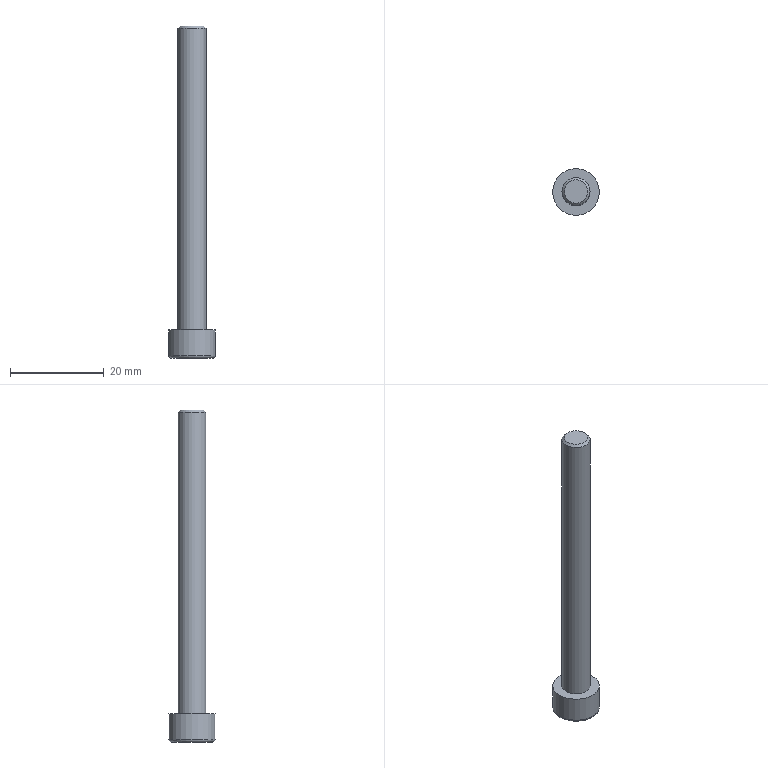Part | NX | features solid 2 | 1 solid | 14 faces | box 10 x 10 x 71 mm | volume 2240 mm3 | plane 10 | cylinder 2 | torus 1 | cone 1 | commonest cylinder face diameters 6 x1 10 x1
STEP:
#1=CARTESIAN_POINT('',(-100.557,-105.5,-189.5));
#2=VERTEX_POINT('',#1);
#3=CARTESIAN_POINT('',(-99.113,-108.,-189.5));
#4=VERTEX_POINT('',#3);
#5=CARTESIAN_POINT('',(-100.557,-105.5,-189.5));
#6=DIRECTION('',(0.5,-0.866,0.));
#7=VECTOR('',#6,1000.);
#8=LINE('',#5,#7);
#9=EDGE_CURVE('',#2,#4,#8,.T.);
#10=ORIENTED_EDGE('',*,*,#9,.F.);
#11=CARTESIAN_POINT('',(-103.443,-105.5,-189.5));
#12=VERTEX_POINT('',#11);
#13=CARTESIAN_POINT('',(-103.443,-105.5,-189.5));
#14=DIRECTION('',(1.,0.,0.));
#15=VECTOR('',#14,1000.);
#16=LINE('',#13,#15);
#17=EDGE_CURVE('',#12,#2,#16,.T.);
#18=ORIENTED_EDGE('',*,*,#17,.F.);
#19=CARTESIAN_POINT('',(-104.887,-108.,-189.5));
#20=VERTEX_POINT('',#19);
#21=CARTESIAN_POINT('',(-104.887,-108.,-189.5));
#22=DIRECTION('',(0.5,0.866,0.));
#23=VECTOR('',#22,1000.);
#24=LINE('',#21,#23);
#25=EDGE_CURVE('',#20,#12,#24,.T.);
#26=ORIENTED_EDGE('',*,*,#25,.F.);
#27=CARTESIAN_POINT('',(-103.443,-110.5,-189.5));
#28=VERTEX_POINT('',#27);
#29=CARTESIAN_POINT('',(-103.443,-110.5,-189.5));
#30=DIRECTION('',(-0.5,0.866,0.));
#31=VECTOR('',#30,1000.);
#32=LINE('',#29,#31);
#33=EDGE_CURVE('',#28,#20,#32,.T.);
#34=ORIENTED_EDGE('',*,*,#33,.F.);
#35=CARTESIAN_POINT('',(-100.557,-110.5,-189.5));
#36=VERTEX_POINT('',#35);
#37=CARTESIAN_POINT('',(-100.557,-110.5,-189.5));
#38=DIRECTION('',(-1.,0.,0.));
#39=VECTOR('',#38,1000.);
#40=LINE('',#37,#39);
#41=EDGE_CURVE('',#36,#28,#40,.T.);
#42=ORIENTED_EDGE('',*,*,#41,.F.);
#43=CARTESIAN_POINT('',(-99.113,-108.,-189.5));
#44=DIRECTION('',(-0.5,-0.866,0.));
#45=VECTOR('',#44,1000.);
#46=LINE('',#43,#45);
#47=EDGE_CURVE('',#4,#36,#46,.T.);
#48=ORIENTED_EDGE('',*,*,#47,.F.);
#49=EDGE_LOOP('',(#10,#18,#26,#34,#42,#48));
#50=FACE_BOUND('',#49,.T.);
#51=CARTESIAN_POINT('',(-106.5,-108.,-189.5));
#52=VERTEX_POINT('',#51);
#53=CARTESIAN_POINT('',(-102.,-108.,-189.5));
#54=DIRECTION('',(0.,0.,-1.));
#55=DIRECTION('',(-1.,0.,0.));
#56=AXIS2_PLACEMENT_3D('',#53,#54,#55);
#57=CIRCLE('',#56,4.5);
#58=EDGE_CURVE('',#52,#52,#57,.T.);
#59=ORIENTED_EDGE('',*,*,#58,.T.);
#60=EDGE_LOOP('',(#59));
#61=FACE_BOUND('',#60,.T.);
#62=CARTESIAN_POINT('',(-102.,-108.,-189.5));
#63=DIRECTION('',(0.,0.,-1.));
#64=DIRECTION('',(-1.,0.,0.));
#65=AXIS2_PLACEMENT_3D('',#62,#63,#64);
#66=PLANE('',#65);
#67=ADVANCED_FACE('',(#50,#61),#66,.T.);
#68=CARTESIAN_POINT('',(-99.,-108.,-183.5));
#69=VERTEX_POINT('',#68);
#70=CARTESIAN_POINT('',(-102.,-108.,-183.5));
#71=DIRECTION('',(0.,0.,1.));
#72=DIRECTION('',(1.,0.,0.));
#73=AXIS2_PLACEMENT_3D('',#70,#71,#72);
#74=CIRCLE('',#73,3.);
#75=EDGE_CURVE('',#69,#69,#74,.T.);
#76=ORIENTED_EDGE('',*,*,#75,.F.);
#77=EDGE_LOOP('',(#76));
#78=FACE_BOUND('',#77,.T.);
#79=CARTESIAN_POINT('',(-97.,-108.,-183.5));
#80=VERTEX_POINT('',#79);
#81=CARTESIAN_POINT('',(-102.,-108.,-183.5));
#82=DIRECTION('',(0.,0.,-1.));
#83=DIRECTION('',(1.,0.,0.));
#84=AXIS2_PLACEMENT_3D('',#81,#82,#83);
#85=CIRCLE('',#84,5.);
#86=EDGE_CURVE('',#80,#80,#85,.T.);
#87=ORIENTED_EDGE('',*,*,#86,.F.);
#88=EDGE_LOOP('',(#87));
#89=FACE_BOUND('',#88,.T.);
#90=CARTESIAN_POINT('',(-102.,-108.,-183.5));
#91=DIRECTION('',(0.,0.,1.));
#92=DIRECTION('',(1.,0.,0.));
#93=AXIS2_PLACEMENT_3D('',#90,#91,#92);
#94=PLANE('',#93);
#95=ADVANCED_FACE('',(#78,#89),#94,.T.);
#96=CARTESIAN_POINT('',(-107.,-108.,-189.));
#97=VERTEX_POINT('',#96);
#98=CARTESIAN_POINT('',(-102.,-108.,-189.));
#99=DIRECTION('',(0.,0.,-1.));
#100=DIRECTION('',(-1.,0.,0.));
#101=AXIS2_PLACEMENT_3D('',#98,#99,#100);
#102=CIRCLE('',#101,5.);
#103=EDGE_CURVE('',#97,#97,#102,.F.);
#104=ORIENTED_EDGE('',*,*,#103,.T.);
#105=EDGE_LOOP('',(#104));
#106=FACE_BOUND('',#105,.T.);
#107=ORIENTED_EDGE('',*,*,#86,.T.);
#108=EDGE_LOOP('',(#107));
#109=FACE_BOUND('',#108,.T.);
#110=CARTESIAN_POINT('',(-102.,-108.,-183.5));
#111=DIRECTION('',(0.,0.,-1.));
#112=DIRECTION('',(1.,0.,0.));
#113=AXIS2_PLACEMENT_3D('',#110,#111,#112);
#114=CYLINDRICAL_SURFACE('',#113,5.);
#115=ADVANCED_FACE('',(#106,#109),#114,.T.);
#116=ORIENTED_EDGE('',*,*,#58,.F.);
#117=EDGE_LOOP('',(#116));
#118=FACE_BOUND('',#117,.T.);
#119=ORIENTED_EDGE('',*,*,#103,.F.);
#120=EDGE_LOOP('',(#119));
#121=FACE_BOUND('',#120,.T.);
#122=CARTESIAN_POINT('',(-102.,-108.,-189.));
#123=DIRECTION('',(0.,0.,-1.));
#124=DIRECTION('',(-1.,0.,0.));
#125=AXIS2_PLACEMENT_3D('',#122,#123,#124);
#126=TOROIDAL_SURFACE('',#125,4.5,0.5);
#127=ADVANCED_FACE('',(#118,#121),#126,.T.);
#128=CARTESIAN_POINT('',(-99.5,-108.,-118.5));
#129=VERTEX_POINT('',#128);
#130=CARTESIAN_POINT('',(-102.,-108.,-118.5));
#131=DIRECTION('',(0.,0.,1.));
#132=DIRECTION('',(1.,0.,0.));
#133=AXIS2_PLACEMENT_3D('',#130,#131,#132);
#134=CIRCLE('',#133,2.5);
#135=EDGE_CURVE('',#129,#129,#134,.T.);
#136=ORIENTED_EDGE('',*,*,#135,.T.);
#137=EDGE_LOOP('',(#136));
#138=FACE_BOUND('',#137,.T.);
#139=CARTESIAN_POINT('',(-102.,-108.,-118.5));
#140=DIRECTION('',(0.,0.,1.));
#141=DIRECTION('',(1.,0.,0.));
#142=AXIS2_PLACEMENT_3D('',#139,#140,#141);
#143=PLANE('',#142);
#144=ADVANCED_FACE('',(#138),#143,.T.);
#145=CARTESIAN_POINT('',(-99.,-108.,-119.));
#146=VERTEX_POINT('',#145);
#147=CARTESIAN_POINT('',(-102.,-108.,-119.));
#148=DIRECTION('',(0.,0.,1.));
#149=DIRECTION('',(1.,0.,0.));
#150=AXIS2_PLACEMENT_3D('',#147,#148,#149);
#151=CIRCLE('',#150,3.);
#152=EDGE_CURVE('',#146,#146,#151,.F.);
#153=ORIENTED_EDGE('',*,*,#152,.T.);
#154=EDGE_LOOP('',(#153));
#155=FACE_BOUND('',#154,.T.);
#156=ORIENTED_EDGE('',*,*,#75,.T.);
#157=EDGE_LOOP('',(#156));
#158=FACE_BOUND('',#157,.T.);
#159=CARTESIAN_POINT('',(-102.,-108.,-118.5));
#160=DIRECTION('',(0.,0.,-1.));
#161=DIRECTION('',(1.,0.,0.));
#162=AXIS2_PLACEMENT_3D('',#159,#160,#161);
#163=CYLINDRICAL_SURFACE('',#162,3.);
#164=ADVANCED_FACE('',(#155,#158),#163,.T.);
#165=ORIENTED_EDGE('',*,*,#135,.F.);
#166=EDGE_LOOP('',(#165));
#167=FACE_BOUND('',#166,.T.);
#168=ORIENTED_EDGE('',*,*,#152,.F.);
#169=EDGE_LOOP('',(#168));
#170=FACE_BOUND('',#169,.T.);
#171=CARTESIAN_POINT('',(-102.,-108.,-119.));
#172=DIRECTION('',(0.,0.,-1.));
#173=DIRECTION('',(-1.,0.,0.));
#174=AXIS2_PLACEMENT_3D('',#171,#172,#173);
#175=CONICAL_SURFACE('',#174,3.,0.7854);
#176=ADVANCED_FACE('',(#167,#170),#175,.T.);
#177=ORIENTED_EDGE('',*,*,#9,.T.);
#178=CARTESIAN_POINT('',(-99.113,-108.,-186.5));
#179=VERTEX_POINT('',#178);
#180=CARTESIAN_POINT('',(-99.113,-108.,-186.5));
#181=DIRECTION('',(0.,0.,-1.));
#182=VECTOR('',#181,1000.);
#183=LINE('',#180,#182);
#184=EDGE_CURVE('',#179,#4,#183,.T.);
#185=ORIENTED_EDGE('',*,*,#184,.F.);
#186=CARTESIAN_POINT('',(-100.557,-105.5,-186.5));
#187=VERTEX_POINT('',#186);
#188=CARTESIAN_POINT('',(-100.557,-105.5,-186.5));
#189=DIRECTION('',(0.5,-0.866,0.));
#190=VECTOR('',#189,1000.);
#191=LINE('',#188,#190);
#192=EDGE_CURVE('',#187,#179,#191,.T.);
#193=ORIENTED_EDGE('',*,*,#192,.F.);
#194=CARTESIAN_POINT('',(-100.557,-105.5,-186.5));
#195=DIRECTION('',(0.,0.,-1.));
#196=VECTOR('',#195,1000.);
#197=LINE('',#194,#196);
#198=EDGE_CURVE('',#187,#2,#197,.T.);
#199=ORIENTED_EDGE('',*,*,#198,.T.);
#200=EDGE_LOOP('',(#177,#185,#193,#199));
#201=FACE_BOUND('',#200,.T.);
#202=CARTESIAN_POINT('',(-99.835,-106.75,-188.));
#203=DIRECTION('',(0.866,0.5,0.));
#204=DIRECTION('',(-0.5,0.866,0.));
#205=AXIS2_PLACEMENT_3D('',#202,#203,#204);
#206=PLANE('',#205);
#207=ADVANCED_FACE('',(#201),#206,.F.);
#208=ORIENTED_EDGE('',*,*,#17,.T.);
#209=ORIENTED_EDGE('',*,*,#198,.F.);
#210=CARTESIAN_POINT('',(-103.443,-105.5,-186.5));
#211=VERTEX_POINT('',#210);
#212=CARTESIAN_POINT('',(-103.443,-105.5,-186.5));
#213=DIRECTION('',(1.,0.,0.));
#214=VECTOR('',#213,1000.);
#215=LINE('',#212,#214);
#216=EDGE_CURVE('',#211,#187,#215,.T.);
#217=ORIENTED_EDGE('',*,*,#216,.F.);
#218=CARTESIAN_POINT('',(-103.443,-105.5,-186.5));
#219=DIRECTION('',(0.,0.,-1.));
#220=VECTOR('',#219,1000.);
#221=LINE('',#218,#220);
#222=EDGE_CURVE('',#211,#12,#221,.T.);
#223=ORIENTED_EDGE('',*,*,#222,.T.);
#224=EDGE_LOOP('',(#208,#209,#217,#223));
#225=FACE_BOUND('',#224,.T.);
#226=CARTESIAN_POINT('',(-102.,-105.5,-188.));
#227=DIRECTION('',(0.,1.,0.));
#228=DIRECTION('',(0.,0.,1.));
#229=AXIS2_PLACEMENT_3D('',#226,#227,#228);
#230=PLANE('',#229);
#231=ADVANCED_FACE('',(#225),#230,.F.);
#232=ORIENTED_EDGE('',*,*,#25,.T.);
#233=ORIENTED_EDGE('',*,*,#222,.F.);
#234=CARTESIAN_POINT('',(-104.887,-108.,-186.5));
#235=VERTEX_POINT('',#234);
#236=CARTESIAN_POINT('',(-104.887,-108.,-186.5));
#237=DIRECTION('',(0.5,0.866,0.));
#238=VECTOR('',#237,1000.);
#239=LINE('',#236,#238);
#240=EDGE_CURVE('',#235,#211,#239,.T.);
#241=ORIENTED_EDGE('',*,*,#240,.F.);
#242=CARTESIAN_POINT('',(-104.887,-108.,-186.5));
#243=DIRECTION('',(0.,0.,-1.));
#244=VECTOR('',#243,1000.);
#245=LINE('',#242,#244);
#246=EDGE_CURVE('',#235,#20,#245,.T.);
#247=ORIENTED_EDGE('',*,*,#246,.T.);
#248=EDGE_LOOP('',(#232,#233,#241,#247));
#249=FACE_BOUND('',#248,.T.);
#250=CARTESIAN_POINT('',(-104.165,-106.75,-188.));
#251=DIRECTION('',(-0.866,0.5,0.));
#252=DIRECTION('',(-0.5,-0.866,0.));
#253=AXIS2_PLACEMENT_3D('',#250,#251,#252);
#254=PLANE('',#253);
#255=ADVANCED_FACE('',(#249),#254,.F.);
#256=ORIENTED_EDGE('',*,*,#33,.T.);
#257=ORIENTED_EDGE('',*,*,#246,.F.);
#258=CARTESIAN_POINT('',(-103.443,-110.5,-186.5));
#259=VERTEX_POINT('',#258);
#260=CARTESIAN_POINT('',(-103.443,-110.5,-186.5));
#261=DIRECTION('',(-0.5,0.866,0.));
#262=VECTOR('',#261,1000.);
#263=LINE('',#260,#262);
#264=EDGE_CURVE('',#259,#235,#263,.T.);
#265=ORIENTED_EDGE('',*,*,#264,.F.);
#266=CARTESIAN_POINT('',(-103.443,-110.5,-186.5));
#267=DIRECTION('',(0.,0.,-1.));
#268=VECTOR('',#267,1000.);
#269=LINE('',#266,#268);
#270=EDGE_CURVE('',#259,#28,#269,.T.);
#271=ORIENTED_EDGE('',*,*,#270,.T.);
#272=EDGE_LOOP('',(#256,#257,#265,#271));
#273=FACE_BOUND('',#272,.T.);
#274=CARTESIAN_POINT('',(-104.165,-109.25,-188.));
#275=DIRECTION('',(-0.866,-0.5,0.));
#276=DIRECTION('',(0.5,-0.866,0.));
#277=AXIS2_PLACEMENT_3D('',#274,#275,#276);
#278=PLANE('',#277);
#279=ADVANCED_FACE('',(#273),#278,.F.);
#280=ORIENTED_EDGE('',*,*,#41,.T.);
#281=ORIENTED_EDGE('',*,*,#270,.F.);
#282=CARTESIAN_POINT('',(-100.557,-110.5,-186.5));
#283=VERTEX_POINT('',#282);
#284=CARTESIAN_POINT('',(-100.557,-110.5,-186.5));
#285=DIRECTION('',(-1.,0.,0.));
#286=VECTOR('',#285,1000.);
#287=LINE('',#284,#286);
#288=EDGE_CURVE('',#283,#259,#287,.T.);
#289=ORIENTED_EDGE('',*,*,#288,.F.);
#290=CARTESIAN_POINT('',(-100.557,-110.5,-186.5));
#291=DIRECTION('',(0.,0.,-1.));
#292=VECTOR('',#291,1000.);
#293=LINE('',#290,#292);
#294=EDGE_CURVE('',#283,#36,#293,.T.);
#295=ORIENTED_EDGE('',*,*,#294,.T.);
#296=EDGE_LOOP('',(#280,#281,#289,#295));
#297=FACE_BOUND('',#296,.T.);
#298=CARTESIAN_POINT('',(-102.,-110.5,-188.));
#299=DIRECTION('',(0.,-1.,0.));
#300=DIRECTION('',(0.,0.,-1.));
#301=AXIS2_PLACEMENT_3D('',#298,#299,#300);
#302=PLANE('',#301);
#303=ADVANCED_FACE('',(#297),#302,.F.);
#304=ORIENTED_EDGE('',*,*,#47,.T.);
#305=ORIENTED_EDGE('',*,*,#294,.F.);
#306=CARTESIAN_POINT('',(-99.113,-108.,-186.5));
#307=DIRECTION('',(-0.5,-0.866,0.));
#308=VECTOR('',#307,1000.);
#309=LINE('',#306,#308);
#310=EDGE_CURVE('',#179,#283,#309,.T.);
#311=ORIENTED_EDGE('',*,*,#310,.F.);
#312=ORIENTED_EDGE('',*,*,#184,.T.);
#313=EDGE_LOOP('',(#304,#305,#311,#312));
#314=FACE_BOUND('',#313,.T.);
#315=CARTESIAN_POINT('',(-99.835,-109.25,-188.));
#316=DIRECTION('',(0.866,-0.5,0.));
#317=DIRECTION('',(0.5,0.866,0.));
#318=AXIS2_PLACEMENT_3D('',#315,#316,#317);
#319=PLANE('',#318);
#320=ADVANCED_FACE('',(#314),#319,.F.);
#321=ORIENTED_EDGE('',*,*,#310,.T.);
#322=ORIENTED_EDGE('',*,*,#288,.T.);
#323=ORIENTED_EDGE('',*,*,#264,.T.);
#324=ORIENTED_EDGE('',*,*,#240,.T.);
#325=ORIENTED_EDGE('',*,*,#216,.T.);
#326=ORIENTED_EDGE('',*,*,#192,.T.);
#327=EDGE_LOOP('',(#321,#322,#323,#324,#325,#326));
#328=FACE_BOUND('',#327,.T.);
#329=CARTESIAN_POINT('',(-102.,-108.,-186.5));
#330=DIRECTION('',(0.,0.,1.));
#331=DIRECTION('',(1.,0.,0.));
#332=AXIS2_PLACEMENT_3D('',#329,#330,#331);
#333=PLANE('',#332);
#334=ADVANCED_FACE('',(#328),#333,.F.);
#335=CLOSED_SHELL('',(#67,#95,#115,#127,#144,#164,#176,#207,#231,#255,#279,#303,#320,#334));
#336=MANIFOLD_SOLID_BREP('',#335);
#337=(LENGTH_UNIT()NAMED_UNIT(*)SI_UNIT(.MILLI.,.METRE.));
#338=UNCERTAINTY_MEASURE_WITH_UNIT(LENGTH_MEASURE(0.00001),#337,'','');
#339=(NAMED_UNIT(*)PLANE_ANGLE_UNIT()SI_UNIT($,.RADIAN.));
#340=(NAMED_UNIT(*)SI_UNIT($,.STERADIAN.)SOLID_ANGLE_UNIT());
#341=(GEOMETRIC_REPRESENTATION_CONTEXT(3)GLOBAL_UNCERTAINTY_ASSIGNED_CONTEXT((#338))GLOBAL_UNIT_ASSIGNED_CONTEXT((#337,#339,#340))REPRESENTATION_CONTEXT('',''));
#342=ADVANCED_BREP_SHAPE_REPRESENTATION('',(#336),#341);